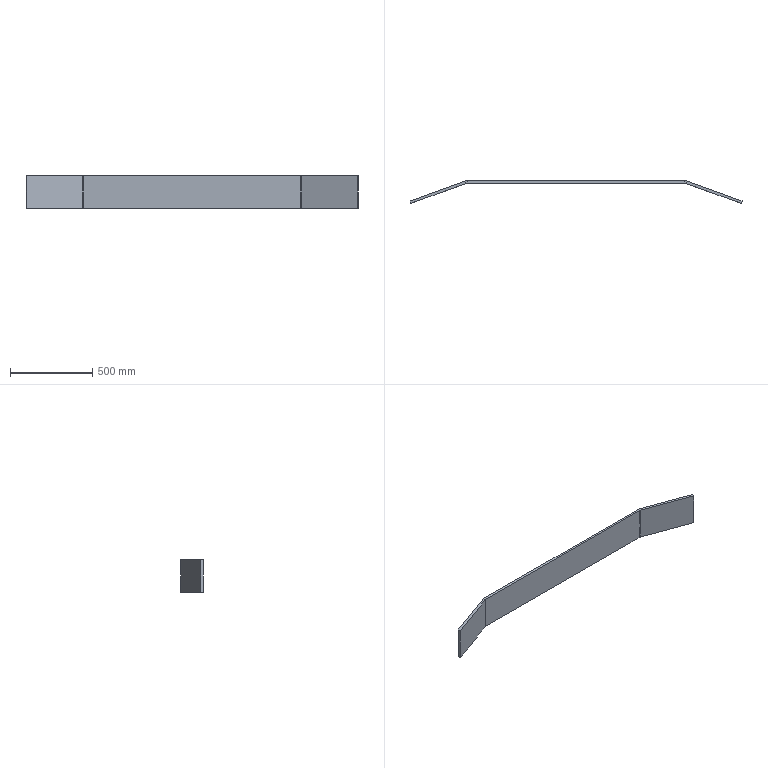Part | SolidWorks | features FlatPattern 1, SMBaseFlange 1, SheetMetal 1 | 1 solid | 22 faces | box 2017 x 139.101 x 200 mm | volume 6576544 mm3 | plane 18 | cylinder 4 | commonest cylinder face diameters 30 x2 62 x2
STEP:
#1=CARTESIAN_POINT('',(672.881,-269.87,200.));
#2=VERTEX_POINT('',#1);
#3=CARTESIAN_POINT('',(667.409,-284.905,200.));
#4=VERTEX_POINT('',#3);
#5=CARTESIAN_POINT('',(672.881,-269.87,200.));
#6=DIRECTION('',(-0.342,-0.9397,0.));
#7=VECTOR('',#6,1000.);
#8=LINE('',#5,#7);
#9=EDGE_CURVE('',#2,#4,#8,.T.);
#10=ORIENTED_EDGE('',*,*,#9,.F.);
#11=CARTESIAN_POINT('',(662.278,-268.,200.));
#12=VERTEX_POINT('',#11);
#13=CARTESIAN_POINT('',(662.278,-299.,200.));
#14=DIRECTION('',(0.,0.,1.));
#15=DIRECTION('',(-1.,0.,0.));
#16=AXIS2_PLACEMENT_3D('',#13,#14,#15);
#17=CIRCLE('',#16,31.);
#18=EDGE_CURVE('',#2,#12,#17,.T.);
#19=ORIENTED_EDGE('',*,*,#18,.T.);
#20=CARTESIAN_POINT('',(662.278,-284.,200.));
#21=VERTEX_POINT('',#20);
#22=CARTESIAN_POINT('',(662.278,-284.,200.));
#23=DIRECTION('',(0.,1.,0.));
#24=VECTOR('',#23,1000.);
#25=LINE('',#22,#24);
#26=EDGE_CURVE('',#21,#12,#25,.T.);
#27=ORIENTED_EDGE('',*,*,#26,.F.);
#28=CARTESIAN_POINT('',(662.278,-299.,200.));
#29=DIRECTION('',(0.,0.,1.));
#30=DIRECTION('',(1.,0.,0.));
#31=AXIS2_PLACEMENT_3D('',#28,#29,#30);
#32=CIRCLE('',#31,15.);
#33=EDGE_CURVE('',#4,#21,#32,.T.);
#34=ORIENTED_EDGE('',*,*,#33,.F.);
#35=EDGE_LOOP('',(#10,#19,#27,#34));
#36=FACE_OUTER_BOUND('',#35,.T.);
#37=CARTESIAN_POINT('',(672.881,-269.87,200.));
#38=DIRECTION('',(0.,0.,1.));
#39=DIRECTION('',(1.,0.,0.));
#40=AXIS2_PLACEMENT_3D('',#37,#38,#39);
#41=PLANE('',#40);
#42=ADVANCED_FACE('',(#36),#41,.T.);
#43=CARTESIAN_POINT('',(1008.613,-392.066,200.));
#44=VERTEX_POINT('',#43);
#45=CARTESIAN_POINT('',(667.744,-268.,200.));
#46=DIRECTION('',(-0.9397,0.342,0.));
#47=VECTOR('',#46,1000.);
#48=LINE('',#45,#47);
#49=EDGE_CURVE('',#44,#2,#48,.T.);
#50=ORIENTED_EDGE('',*,*,#49,.T.);
#51=ORIENTED_EDGE('',*,*,#9,.T.);
#52=CARTESIAN_POINT('',(1003.14,-407.101,200.));
#53=VERTEX_POINT('',#52);
#54=CARTESIAN_POINT('',(662.272,-283.035,200.));
#55=DIRECTION('',(-0.9397,0.342,0.));
#56=VECTOR('',#55,1000.);
#57=LINE('',#54,#56);
#58=EDGE_CURVE('',#53,#4,#57,.T.);
#59=ORIENTED_EDGE('',*,*,#58,.F.);
#60=CARTESIAN_POINT('',(1008.613,-392.066,200.));
#61=DIRECTION('',(-0.342,-0.9397,0.));
#62=VECTOR('',#61,1000.);
#63=LINE('',#60,#62);
#64=EDGE_CURVE('',#44,#53,#63,.T.);
#65=ORIENTED_EDGE('',*,*,#64,.F.);
#66=EDGE_LOOP('',(#50,#51,#59,#65));
#67=FACE_OUTER_BOUND('',#66,.T.);
#68=CARTESIAN_POINT('',(662.278,-284.,200.));
#69=DIRECTION('',(0.,0.,1.));
#70=DIRECTION('',(1.,0.,0.));
#71=AXIS2_PLACEMENT_3D('',#68,#69,#70);
#72=PLANE('',#71);
#73=ADVANCED_FACE('',(#67),#72,.T.);
#74=CARTESIAN_POINT('',(662.278,-268.,0.));
#75=VERTEX_POINT('',#74);
#76=CARTESIAN_POINT('',(662.278,-284.,0.));
#77=VERTEX_POINT('',#76);
#78=CARTESIAN_POINT('',(662.278,-268.,0.));
#79=DIRECTION('',(0.,-1.,0.));
#80=VECTOR('',#79,1000.);
#81=LINE('',#78,#80);
#82=EDGE_CURVE('',#75,#77,#81,.T.);
#83=ORIENTED_EDGE('',*,*,#82,.F.);
#84=CARTESIAN_POINT('',(672.881,-269.87,0.));
#85=VERTEX_POINT('',#84);
#86=CARTESIAN_POINT('',(662.278,-299.,0.));
#87=DIRECTION('',(0.,0.,1.));
#88=DIRECTION('',(-1.,0.,0.));
#89=AXIS2_PLACEMENT_3D('',#86,#87,#88);
#90=CIRCLE('',#89,31.);
#91=EDGE_CURVE('',#85,#75,#90,.T.);
#92=ORIENTED_EDGE('',*,*,#91,.F.);
#93=CARTESIAN_POINT('',(667.409,-284.905,0.));
#94=VERTEX_POINT('',#93);
#95=CARTESIAN_POINT('',(667.409,-284.905,0.));
#96=DIRECTION('',(0.342,0.9397,0.));
#97=VECTOR('',#96,1000.);
#98=LINE('',#95,#97);
#99=EDGE_CURVE('',#94,#85,#98,.T.);
#100=ORIENTED_EDGE('',*,*,#99,.F.);
#101=CARTESIAN_POINT('',(662.278,-299.,0.));
#102=DIRECTION('',(0.,0.,1.));
#103=DIRECTION('',(1.,0.,0.));
#104=AXIS2_PLACEMENT_3D('',#101,#102,#103);
#105=CIRCLE('',#104,15.);
#106=EDGE_CURVE('',#94,#77,#105,.T.);
#107=ORIENTED_EDGE('',*,*,#106,.T.);
#108=EDGE_LOOP('',(#83,#92,#100,#107));
#109=FACE_OUTER_BOUND('',#108,.T.);
#110=CARTESIAN_POINT('',(662.278,-268.,0.));
#111=DIRECTION('',(0.,0.,-1.));
#112=DIRECTION('',(-1.,0.,0.));
#113=AXIS2_PLACEMENT_3D('',#110,#111,#112);
#114=PLANE('',#113);
#115=ADVANCED_FACE('',(#109),#114,.T.);
#116=CARTESIAN_POINT('',(-662.278,-268.,0.));
#117=VERTEX_POINT('',#116);
#118=CARTESIAN_POINT('',(-667.744,-268.,0.));
#119=DIRECTION('',(-1.,0.,0.));
#120=VECTOR('',#119,1000.);
#121=LINE('',#118,#120);
#122=EDGE_CURVE('',#75,#117,#121,.T.);
#123=ORIENTED_EDGE('',*,*,#122,.F.);
#124=ORIENTED_EDGE('',*,*,#82,.T.);
#125=CARTESIAN_POINT('',(-662.278,-284.,0.));
#126=VERTEX_POINT('',#125);
#127=CARTESIAN_POINT('',(-667.744,-284.,0.));
#128=DIRECTION('',(-1.,0.,0.));
#129=VECTOR('',#128,1000.);
#130=LINE('',#127,#129);
#131=EDGE_CURVE('',#77,#126,#130,.T.);
#132=ORIENTED_EDGE('',*,*,#131,.T.);
#133=CARTESIAN_POINT('',(-662.278,-284.,0.));
#134=DIRECTION('',(0.,1.,0.));
#135=VECTOR('',#134,1000.);
#136=LINE('',#133,#135);
#137=EDGE_CURVE('',#126,#117,#136,.T.);
#138=ORIENTED_EDGE('',*,*,#137,.T.);
#139=EDGE_LOOP('',(#123,#124,#132,#138));
#140=FACE_OUTER_BOUND('',#139,.T.);
#141=CARTESIAN_POINT('',(667.409,-284.905,0.));
#142=DIRECTION('',(0.,0.,-1.));
#143=DIRECTION('',(-1.,0.,0.));
#144=AXIS2_PLACEMENT_3D('',#141,#142,#143);
#145=PLANE('',#144);
#146=ADVANCED_FACE('',(#140),#145,.T.);
#147=CARTESIAN_POINT('',(-662.278,-268.,200.));
#148=VERTEX_POINT('',#147);
#149=CARTESIAN_POINT('',(-662.278,-284.,200.));
#150=VERTEX_POINT('',#149);
#151=CARTESIAN_POINT('',(-662.278,-268.,200.));
#152=DIRECTION('',(0.,-1.,0.));
#153=VECTOR('',#152,1000.);
#154=LINE('',#151,#153);
#155=EDGE_CURVE('',#148,#150,#154,.T.);
#156=ORIENTED_EDGE('',*,*,#155,.F.);
#157=CARTESIAN_POINT('',(-672.881,-269.87,200.));
#158=VERTEX_POINT('',#157);
#159=CARTESIAN_POINT('',(-662.278,-299.,200.));
#160=DIRECTION('',(0.,0.,1.));
#161=DIRECTION('',(-1.,0.,0.));
#162=AXIS2_PLACEMENT_3D('',#159,#160,#161);
#163=CIRCLE('',#162,31.);
#164=EDGE_CURVE('',#148,#158,#163,.T.);
#165=ORIENTED_EDGE('',*,*,#164,.T.);
#166=CARTESIAN_POINT('',(-667.409,-284.905,200.));
#167=VERTEX_POINT('',#166);
#168=CARTESIAN_POINT('',(-667.409,-284.905,200.));
#169=DIRECTION('',(-0.342,0.9397,0.));
#170=VECTOR('',#169,1000.);
#171=LINE('',#168,#170);
#172=EDGE_CURVE('',#167,#158,#171,.T.);
#173=ORIENTED_EDGE('',*,*,#172,.F.);
#174=CARTESIAN_POINT('',(-662.278,-299.,200.));
#175=DIRECTION('',(0.,0.,1.));
#176=DIRECTION('',(1.,0.,0.));
#177=AXIS2_PLACEMENT_3D('',#174,#175,#176);
#178=CIRCLE('',#177,15.);
#179=EDGE_CURVE('',#150,#167,#178,.T.);
#180=ORIENTED_EDGE('',*,*,#179,.F.);
#181=EDGE_LOOP('',(#156,#165,#173,#180));
#182=FACE_OUTER_BOUND('',#181,.T.);
#183=CARTESIAN_POINT('',(-662.278,-268.,200.));
#184=DIRECTION('',(0.,0.,1.));
#185=DIRECTION('',(1.,0.,0.));
#186=AXIS2_PLACEMENT_3D('',#183,#184,#185);
#187=PLANE('',#186);
#188=ADVANCED_FACE('',(#182),#187,.T.);
#189=CARTESIAN_POINT('',(-667.744,-268.,200.));
#190=DIRECTION('',(-1.,0.,0.));
#191=VECTOR('',#190,1000.);
#192=LINE('',#189,#191);
#193=EDGE_CURVE('',#12,#148,#192,.T.);
#194=ORIENTED_EDGE('',*,*,#193,.T.);
#195=ORIENTED_EDGE('',*,*,#155,.T.);
#196=CARTESIAN_POINT('',(-667.744,-284.,200.));
#197=DIRECTION('',(-1.,0.,0.));
#198=VECTOR('',#197,1000.);
#199=LINE('',#196,#198);
#200=EDGE_CURVE('',#21,#150,#199,.T.);
#201=ORIENTED_EDGE('',*,*,#200,.F.);
#202=ORIENTED_EDGE('',*,*,#26,.T.);
#203=EDGE_LOOP('',(#194,#195,#201,#202));
#204=FACE_OUTER_BOUND('',#203,.T.);
#205=CARTESIAN_POINT('',(-667.409,-284.905,200.));
#206=DIRECTION('',(0.,0.,1.));
#207=DIRECTION('',(1.,0.,0.));
#208=AXIS2_PLACEMENT_3D('',#205,#206,#207);
#209=PLANE('',#208);
#210=ADVANCED_FACE('',(#204),#209,.T.);
#211=CARTESIAN_POINT('',(-672.881,-269.87,0.));
#212=VERTEX_POINT('',#211);
#213=CARTESIAN_POINT('',(-667.409,-284.905,0.));
#214=VERTEX_POINT('',#213);
#215=CARTESIAN_POINT('',(-672.881,-269.87,0.));
#216=DIRECTION('',(0.342,-0.9397,0.));
#217=VECTOR('',#216,1000.);
#218=LINE('',#215,#217);
#219=EDGE_CURVE('',#212,#214,#218,.T.);
#220=ORIENTED_EDGE('',*,*,#219,.F.);
#221=CARTESIAN_POINT('',(-662.278,-299.,0.));
#222=DIRECTION('',(0.,0.,1.));
#223=DIRECTION('',(-1.,0.,0.));
#224=AXIS2_PLACEMENT_3D('',#221,#222,#223);
#225=CIRCLE('',#224,31.);
#226=EDGE_CURVE('',#117,#212,#225,.T.);
#227=ORIENTED_EDGE('',*,*,#226,.F.);
#228=ORIENTED_EDGE('',*,*,#137,.F.);
#229=CARTESIAN_POINT('',(-662.278,-299.,0.));
#230=DIRECTION('',(0.,0.,1.));
#231=DIRECTION('',(1.,0.,0.));
#232=AXIS2_PLACEMENT_3D('',#229,#230,#231);
#233=CIRCLE('',#232,15.);
#234=EDGE_CURVE('',#126,#214,#233,.T.);
#235=ORIENTED_EDGE('',*,*,#234,.T.);
#236=EDGE_LOOP('',(#220,#227,#228,#235));
#237=FACE_OUTER_BOUND('',#236,.T.);
#238=CARTESIAN_POINT('',(-672.881,-269.87,0.));
#239=DIRECTION('',(0.,0.,-1.));
#240=DIRECTION('',(-1.,0.,0.));
#241=AXIS2_PLACEMENT_3D('',#238,#239,#240);
#242=PLANE('',#241);
#243=ADVANCED_FACE('',(#237),#242,.T.);
#244=CARTESIAN_POINT('',(-1008.613,-392.066,0.));
#245=VERTEX_POINT('',#244);
#246=CARTESIAN_POINT('',(-667.744,-268.,0.));
#247=DIRECTION('',(-0.9397,-0.342,0.));
#248=VECTOR('',#247,1000.);
#249=LINE('',#246,#248);
#250=EDGE_CURVE('',#212,#245,#249,.T.);
#251=ORIENTED_EDGE('',*,*,#250,.F.);
#252=ORIENTED_EDGE('',*,*,#219,.T.);
#253=CARTESIAN_POINT('',(-1003.14,-407.101,0.));
#254=VERTEX_POINT('',#253);
#255=CARTESIAN_POINT('',(-662.272,-283.035,0.));
#256=DIRECTION('',(-0.9397,-0.342,0.));
#257=VECTOR('',#256,1000.);
#258=LINE('',#255,#257);
#259=EDGE_CURVE('',#214,#254,#258,.T.);
#260=ORIENTED_EDGE('',*,*,#259,.T.);
#261=CARTESIAN_POINT('',(-1003.14,-407.101,0.));
#262=DIRECTION('',(-0.342,0.9397,0.));
#263=VECTOR('',#262,1000.);
#264=LINE('',#261,#263);
#265=EDGE_CURVE('',#254,#245,#264,.T.);
#266=ORIENTED_EDGE('',*,*,#265,.T.);
#267=EDGE_LOOP('',(#251,#252,#260,#266));
#268=FACE_OUTER_BOUND('',#267,.T.);
#269=CARTESIAN_POINT('',(-662.278,-284.,0.));
#270=DIRECTION('',(0.,0.,-1.));
#271=DIRECTION('',(-1.,0.,0.));
#272=AXIS2_PLACEMENT_3D('',#269,#270,#271);
#273=PLANE('',#272);
#274=ADVANCED_FACE('',(#268),#273,.T.);
#275=ORIENTED_EDGE('',*,*,#250,.T.);
#276=CARTESIAN_POINT('',(-1008.613,-392.066,200.));
#277=VERTEX_POINT('',#276);
#278=CARTESIAN_POINT('',(-1008.613,-392.066,200.));
#279=DIRECTION('',(0.,0.,-1.));
#280=VECTOR('',#279,1000.);
#281=LINE('',#278,#280);
#282=EDGE_CURVE('',#277,#245,#281,.T.);
#283=ORIENTED_EDGE('',*,*,#282,.F.);
#284=CARTESIAN_POINT('',(-667.744,-268.,200.));
#285=DIRECTION('',(-0.9397,-0.342,0.));
#286=VECTOR('',#285,1000.);
#287=LINE('',#284,#286);
#288=EDGE_CURVE('',#158,#277,#287,.T.);
#289=ORIENTED_EDGE('',*,*,#288,.F.);
#290=CARTESIAN_POINT('',(-672.881,-269.87,200.));
#291=DIRECTION('',(0.,0.,-1.));
#292=VECTOR('',#291,1000.);
#293=LINE('',#290,#292);
#294=EDGE_CURVE('',#158,#212,#293,.T.);
#295=ORIENTED_EDGE('',*,*,#294,.T.);
#296=EDGE_LOOP('',(#275,#283,#289,#295));
#297=FACE_OUTER_BOUND('',#296,.T.);
#298=CARTESIAN_POINT('',(-667.744,-268.,200.));
#299=DIRECTION('',(0.342,-0.9397,0.));
#300=DIRECTION('',(0.9397,0.342,0.));
#301=AXIS2_PLACEMENT_3D('',#298,#299,#300);
#302=PLANE('',#301);
#303=ADVANCED_FACE('',(#297),#302,.F.);
#304=ORIENTED_EDGE('',*,*,#265,.F.);
#305=CARTESIAN_POINT('',(-1003.14,-407.101,200.));
#306=VERTEX_POINT('',#305);
#307=CARTESIAN_POINT('',(-1003.14,-407.101,200.));
#308=DIRECTION('',(0.,0.,-1.));
#309=VECTOR('',#308,1000.);
#310=LINE('',#307,#309);
#311=EDGE_CURVE('',#306,#254,#310,.T.);
#312=ORIENTED_EDGE('',*,*,#311,.F.);
#313=CARTESIAN_POINT('',(-1003.14,-407.101,200.));
#314=DIRECTION('',(-0.342,0.9397,0.));
#315=VECTOR('',#314,1000.);
#316=LINE('',#313,#315);
#317=EDGE_CURVE('',#306,#277,#316,.T.);
#318=ORIENTED_EDGE('',*,*,#317,.T.);
#319=ORIENTED_EDGE('',*,*,#282,.T.);
#320=EDGE_LOOP('',(#304,#312,#318,#319));
#321=FACE_OUTER_BOUND('',#320,.T.);
#322=CARTESIAN_POINT('',(-1003.14,-407.101,200.));
#323=DIRECTION('',(-0.9397,-0.342,0.));
#324=DIRECTION('',(0.342,-0.9397,0.));
#325=AXIS2_PLACEMENT_3D('',#322,#323,#324);
#326=PLANE('',#325);
#327=ADVANCED_FACE('',(#321),#326,.T.);
#328=ORIENTED_EDGE('',*,*,#259,.F.);
#329=CARTESIAN_POINT('',(-667.409,-284.905,200.));
#330=DIRECTION('',(0.,0.,-1.));
#331=VECTOR('',#330,1000.);
#332=LINE('',#329,#331);
#333=EDGE_CURVE('',#167,#214,#332,.T.);
#334=ORIENTED_EDGE('',*,*,#333,.F.);
#335=CARTESIAN_POINT('',(-662.272,-283.035,200.));
#336=DIRECTION('',(-0.9397,-0.342,0.));
#337=VECTOR('',#336,1000.);
#338=LINE('',#335,#337);
#339=EDGE_CURVE('',#167,#306,#338,.T.);
#340=ORIENTED_EDGE('',*,*,#339,.T.);
#341=ORIENTED_EDGE('',*,*,#311,.T.);
#342=EDGE_LOOP('',(#328,#334,#340,#341));
#343=FACE_OUTER_BOUND('',#342,.T.);
#344=CARTESIAN_POINT('',(-662.272,-283.035,200.));
#345=DIRECTION('',(0.342,-0.9397,0.));
#346=DIRECTION('',(0.9397,0.342,0.));
#347=AXIS2_PLACEMENT_3D('',#344,#345,#346);
#348=PLANE('',#347);
#349=ADVANCED_FACE('',(#343),#348,.T.);
#350=ORIENTED_EDGE('',*,*,#234,.F.);
#351=CARTESIAN_POINT('',(-662.278,-284.,200.));
#352=DIRECTION('',(0.,0.,-1.));
#353=VECTOR('',#352,1000.);
#354=LINE('',#351,#353);
#355=EDGE_CURVE('',#150,#126,#354,.T.);
#356=ORIENTED_EDGE('',*,*,#355,.F.);
#357=ORIENTED_EDGE('',*,*,#179,.T.);
#358=ORIENTED_EDGE('',*,*,#333,.T.);
#359=EDGE_LOOP('',(#350,#356,#357,#358));
#360=FACE_OUTER_BOUND('',#359,.T.);
#361=CARTESIAN_POINT('',(-662.278,-299.,200.));
#362=DIRECTION('',(0.,0.,-1.));
#363=DIRECTION('',(-1.,0.,0.));
#364=AXIS2_PLACEMENT_3D('',#361,#362,#363);
#365=CYLINDRICAL_SURFACE('',#364,15.);
#366=ADVANCED_FACE('',(#360),#365,.F.);
#367=ORIENTED_EDGE('',*,*,#131,.F.);
#368=CARTESIAN_POINT('',(662.278,-284.,200.));
#369=DIRECTION('',(0.,0.,-1.));
#370=VECTOR('',#369,1000.);
#371=LINE('',#368,#370);
#372=EDGE_CURVE('',#21,#77,#371,.T.);
#373=ORIENTED_EDGE('',*,*,#372,.F.);
#374=ORIENTED_EDGE('',*,*,#200,.T.);
#375=ORIENTED_EDGE('',*,*,#355,.T.);
#376=EDGE_LOOP('',(#367,#373,#374,#375));
#377=FACE_OUTER_BOUND('',#376,.T.);
#378=CARTESIAN_POINT('',(-667.744,-284.,200.));
#379=DIRECTION('',(0.,-1.,0.));
#380=DIRECTION('',(0.,0.,-1.));
#381=AXIS2_PLACEMENT_3D('',#378,#379,#380);
#382=PLANE('',#381);
#383=ADVANCED_FACE('',(#377),#382,.T.);
#384=ORIENTED_EDGE('',*,*,#106,.F.);
#385=CARTESIAN_POINT('',(667.409,-284.905,200.));
#386=DIRECTION('',(0.,0.,-1.));
#387=VECTOR('',#386,1000.);
#388=LINE('',#385,#387);
#389=EDGE_CURVE('',#4,#94,#388,.T.);
#390=ORIENTED_EDGE('',*,*,#389,.F.);
#391=ORIENTED_EDGE('',*,*,#33,.T.);
#392=ORIENTED_EDGE('',*,*,#372,.T.);
#393=EDGE_LOOP('',(#384,#390,#391,#392));
#394=FACE_OUTER_BOUND('',#393,.T.);
#395=CARTESIAN_POINT('',(662.278,-299.,200.));
#396=DIRECTION('',(0.,0.,-1.));
#397=DIRECTION('',(-1.,0.,0.));
#398=AXIS2_PLACEMENT_3D('',#395,#396,#397);
#399=CYLINDRICAL_SURFACE('',#398,15.);
#400=ADVANCED_FACE('',(#394),#399,.F.);
#401=CARTESIAN_POINT('',(1003.14,-407.101,0.));
#402=VERTEX_POINT('',#401);
#403=CARTESIAN_POINT('',(662.272,-283.035,0.));
#404=DIRECTION('',(-0.9397,0.342,0.));
#405=VECTOR('',#404,1000.);
#406=LINE('',#403,#405);
#407=EDGE_CURVE('',#402,#94,#406,.T.);
#408=ORIENTED_EDGE('',*,*,#407,.F.);
#409=CARTESIAN_POINT('',(1003.14,-407.101,200.));
#410=DIRECTION('',(0.,0.,-1.));
#411=VECTOR('',#410,1000.);
#412=LINE('',#409,#411);
#413=EDGE_CURVE('',#53,#402,#412,.T.);
#414=ORIENTED_EDGE('',*,*,#413,.F.);
#415=ORIENTED_EDGE('',*,*,#58,.T.);
#416=ORIENTED_EDGE('',*,*,#389,.T.);
#417=EDGE_LOOP('',(#408,#414,#415,#416));
#418=FACE_OUTER_BOUND('',#417,.T.);
#419=CARTESIAN_POINT('',(662.272,-283.035,200.));
#420=DIRECTION('',(-0.342,-0.9397,0.));
#421=DIRECTION('',(0.9397,-0.342,0.));
#422=AXIS2_PLACEMENT_3D('',#419,#420,#421);
#423=PLANE('',#422);
#424=ADVANCED_FACE('',(#418),#423,.T.);
#425=CARTESIAN_POINT('',(1008.613,-392.066,0.));
#426=VERTEX_POINT('',#425);
#427=CARTESIAN_POINT('',(1008.613,-392.066,0.));
#428=DIRECTION('',(-0.342,-0.9397,0.));
#429=VECTOR('',#428,1000.);
#430=LINE('',#427,#429);
#431=EDGE_CURVE('',#426,#402,#430,.T.);
#432=ORIENTED_EDGE('',*,*,#431,.F.);
#433=CARTESIAN_POINT('',(1008.613,-392.066,200.));
#434=DIRECTION('',(0.,0.,-1.));
#435=VECTOR('',#434,1000.);
#436=LINE('',#433,#435);
#437=EDGE_CURVE('',#44,#426,#436,.T.);
#438=ORIENTED_EDGE('',*,*,#437,.F.);
#439=ORIENTED_EDGE('',*,*,#64,.T.);
#440=ORIENTED_EDGE('',*,*,#413,.T.);
#441=EDGE_LOOP('',(#432,#438,#439,#440));
#442=FACE_OUTER_BOUND('',#441,.T.);
#443=CARTESIAN_POINT('',(1008.613,-392.066,200.));
#444=DIRECTION('',(0.9397,-0.342,0.));
#445=DIRECTION('',(0.342,0.9397,0.));
#446=AXIS2_PLACEMENT_3D('',#443,#444,#445);
#447=PLANE('',#446);
#448=ADVANCED_FACE('',(#442),#447,.T.);
#449=CARTESIAN_POINT('',(667.744,-268.,0.));
#450=DIRECTION('',(-0.9397,0.342,0.));
#451=VECTOR('',#450,1000.);
#452=LINE('',#449,#451);
#453=EDGE_CURVE('',#426,#85,#452,.T.);
#454=ORIENTED_EDGE('',*,*,#453,.T.);
#455=CARTESIAN_POINT('',(672.881,-269.87,200.));
#456=DIRECTION('',(0.,0.,-1.));
#457=VECTOR('',#456,1000.);
#458=LINE('',#455,#457);
#459=EDGE_CURVE('',#2,#85,#458,.T.);
#460=ORIENTED_EDGE('',*,*,#459,.F.);
#461=ORIENTED_EDGE('',*,*,#49,.F.);
#462=ORIENTED_EDGE('',*,*,#437,.T.);
#463=EDGE_LOOP('',(#454,#460,#461,#462));
#464=FACE_OUTER_BOUND('',#463,.T.);
#465=CARTESIAN_POINT('',(667.744,-268.,200.));
#466=DIRECTION('',(-0.342,-0.9397,0.));
#467=DIRECTION('',(0.9397,-0.342,0.));
#468=AXIS2_PLACEMENT_3D('',#465,#466,#467);
#469=PLANE('',#468);
#470=ADVANCED_FACE('',(#464),#469,.F.);
#471=ORIENTED_EDGE('',*,*,#91,.T.);
#472=CARTESIAN_POINT('',(662.278,-268.,200.));
#473=DIRECTION('',(0.,0.,-1.));
#474=VECTOR('',#473,1000.);
#475=LINE('',#472,#474);
#476=EDGE_CURVE('',#12,#75,#475,.T.);
#477=ORIENTED_EDGE('',*,*,#476,.F.);
#478=ORIENTED_EDGE('',*,*,#18,.F.);
#479=ORIENTED_EDGE('',*,*,#459,.T.);
#480=EDGE_LOOP('',(#471,#477,#478,#479));
#481=FACE_OUTER_BOUND('',#480,.T.);
#482=CARTESIAN_POINT('',(662.278,-299.,200.));
#483=DIRECTION('',(0.,0.,-1.));
#484=DIRECTION('',(-1.,0.,0.));
#485=AXIS2_PLACEMENT_3D('',#482,#483,#484);
#486=CYLINDRICAL_SURFACE('',#485,31.);
#487=ADVANCED_FACE('',(#481),#486,.T.);
#488=ORIENTED_EDGE('',*,*,#122,.T.);
#489=CARTESIAN_POINT('',(-662.278,-268.,200.));
#490=DIRECTION('',(0.,0.,-1.));
#491=VECTOR('',#490,1000.);
#492=LINE('',#489,#491);
#493=EDGE_CURVE('',#148,#117,#492,.T.);
#494=ORIENTED_EDGE('',*,*,#493,.F.);
#495=ORIENTED_EDGE('',*,*,#193,.F.);
#496=ORIENTED_EDGE('',*,*,#476,.T.);
#497=EDGE_LOOP('',(#488,#494,#495,#496));
#498=FACE_OUTER_BOUND('',#497,.T.);
#499=CARTESIAN_POINT('',(-667.744,-268.,200.));
#500=DIRECTION('',(0.,-1.,0.));
#501=DIRECTION('',(0.,0.,-1.));
#502=AXIS2_PLACEMENT_3D('',#499,#500,#501);
#503=PLANE('',#502);
#504=ADVANCED_FACE('',(#498),#503,.F.);
#505=ORIENTED_EDGE('',*,*,#226,.T.);
#506=ORIENTED_EDGE('',*,*,#294,.F.);
#507=ORIENTED_EDGE('',*,*,#164,.F.);
#508=ORIENTED_EDGE('',*,*,#493,.T.);
#509=EDGE_LOOP('',(#505,#506,#507,#508));
#510=FACE_OUTER_BOUND('',#509,.T.);
#511=CARTESIAN_POINT('',(-662.278,-299.,200.));
#512=DIRECTION('',(0.,0.,-1.));
#513=DIRECTION('',(-1.,0.,0.));
#514=AXIS2_PLACEMENT_3D('',#511,#512,#513);
#515=CYLINDRICAL_SURFACE('',#514,31.);
#516=ADVANCED_FACE('',(#510),#515,.T.);
#517=ORIENTED_EDGE('',*,*,#288,.T.);
#518=ORIENTED_EDGE('',*,*,#317,.F.);
#519=ORIENTED_EDGE('',*,*,#339,.F.);
#520=ORIENTED_EDGE('',*,*,#172,.T.);
#521=EDGE_LOOP('',(#517,#518,#519,#520));
#522=FACE_OUTER_BOUND('',#521,.T.);
#523=CARTESIAN_POINT('',(-662.278,-299.,200.));
#524=DIRECTION('',(0.,0.,1.));
#525=DIRECTION('',(1.,0.,0.));
#526=AXIS2_PLACEMENT_3D('',#523,#524,#525);
#527=PLANE('',#526);
#528=ADVANCED_FACE('',(#522),#527,.T.);
#529=ORIENTED_EDGE('',*,*,#407,.T.);
#530=ORIENTED_EDGE('',*,*,#99,.T.);
#531=ORIENTED_EDGE('',*,*,#453,.F.);
#532=ORIENTED_EDGE('',*,*,#431,.T.);
#533=EDGE_LOOP('',(#529,#530,#531,#532));
#534=FACE_OUTER_BOUND('',#533,.T.);
#535=CARTESIAN_POINT('',(-662.278,-299.,0.));
#536=DIRECTION('',(0.,0.,1.));
#537=DIRECTION('',(1.,0.,0.));
#538=AXIS2_PLACEMENT_3D('',#535,#536,#537);
#539=PLANE('',#538);
#540=ADVANCED_FACE('',(#534),#539,.F.);
#541=CLOSED_SHELL('',(#42,#73,#115,#146,#188,#210,#243,#274,#303,#327,#349,#366,#383,#400,#424,#448,#470,#487,#504,#516,#528,#540));
#542=MANIFOLD_SOLID_BREP('',#541);
#543=CARTESIAN_POINT('',(0.,0.,0.));
#544=DIRECTION('',(0.,0.,1.));
#545=DIRECTION('',(1.,0.,0.));
#546=AXIS2_PLACEMENT_3D('',#543,#544,#545);
#547=(LENGTH_UNIT()NAMED_UNIT(*)SI_UNIT(.MILLI.,.METRE.));
#548=UNCERTAINTY_MEASURE_WITH_UNIT(LENGTH_MEASURE(0.00001),#547,'','');
#549=(NAMED_UNIT(*)PLANE_ANGLE_UNIT()SI_UNIT($,.RADIAN.));
#550=(NAMED_UNIT(*)SI_UNIT($,.STERADIAN.)SOLID_ANGLE_UNIT());
#551=(GEOMETRIC_REPRESENTATION_CONTEXT(3)GLOBAL_UNCERTAINTY_ASSIGNED_CONTEXT((#548))GLOBAL_UNIT_ASSIGNED_CONTEXT((#547,#549,#550))REPRESENTATION_CONTEXT('',''));
#552=ADVANCED_BREP_SHAPE_REPRESENTATION('',(#542,#546),#551);